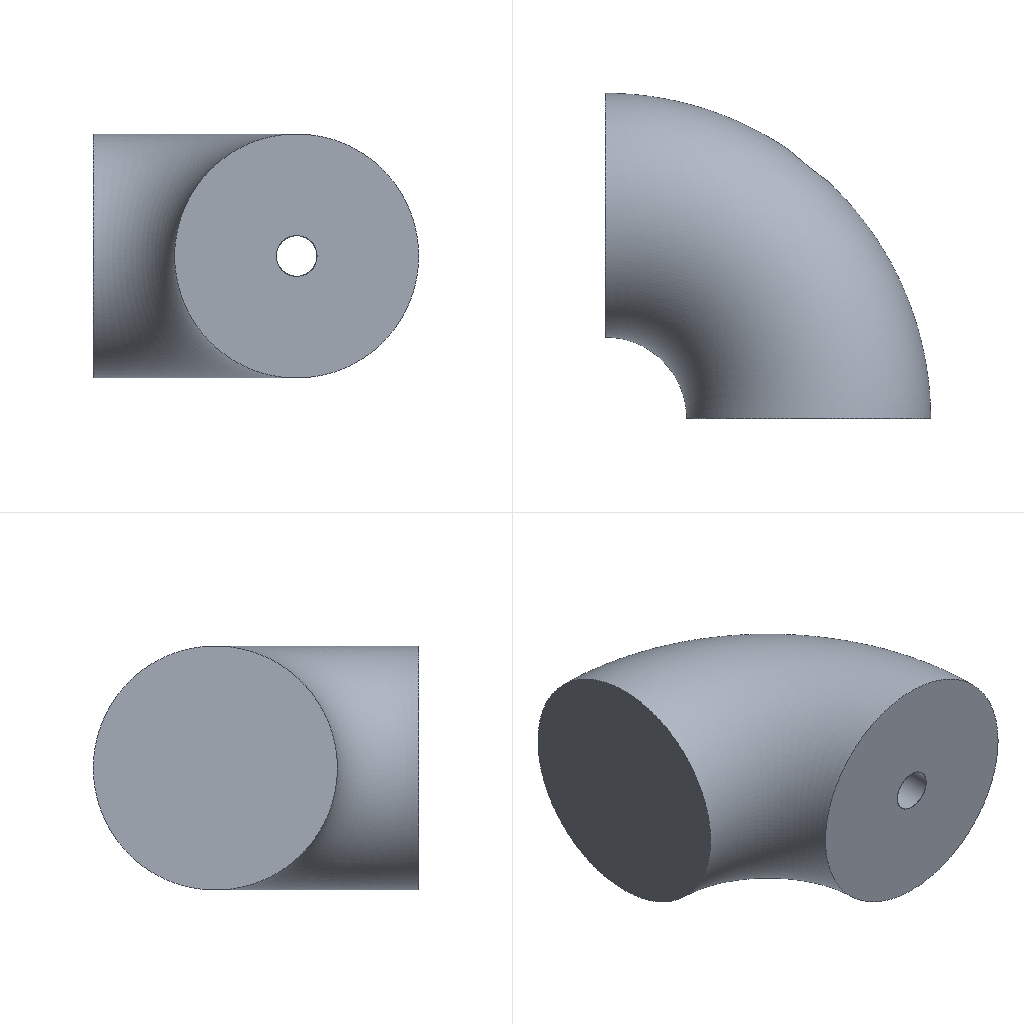Simulation study | ansys fluent
Set-up summary:
category,name,step,type,value,unit,region
solver,ansys_fluent,,Fluent 26.1.0
units,SI m-kg-s (Fluent internal),,stated,boundary values in the units shown in brackets; results in listed units
analysis,deck-1.cas,,cfd steady,"dimension=3D; solver=3d, dp, dbns imp, lam (3d, double precision, density-based implicit, laminar); source_case=2.cas"
model,Space,deck-1.cas,,3D
model,Time,deck-1.cas,,Steady
model,Viscous,deck-1.cas,,Laminar
model,Heat Transfer,deck-1.cas,,Enabled
model,Multiphase,deck-1.cas,,Disabled
analysis,deck-2.cas,,cfd steady,"dimension=3D; solver=3d, dp, dbns imp, lam (3d, double precision, density-based implicit, laminar); source_case=.cas.h5"
model,Space,deck-2.cas,,3D
model,Time,deck-2.cas,,Steady
model,Viscous,deck-2.cas,,Laminar
model,Heat Transfer,deck-2.cas,,Enabled
model,Multiphase,deck-2.cas,,Disabled
mesh,deck-1.cas,,nodes,282132
mesh,deck-1.cas,,elements,266016
mesh,deck-1.cas,,faces,813961
mesh,deck-1.cas,,note,elements = cells; counts from the case file zone headers
mesh,deck-2.cas,,nodes,282132
mesh,deck-2.cas,,elements,266016
mesh,deck-2.cas,,faces,813961
mesh,deck-2.cas,,note,elements = cells; counts from the case file zone headers
cell_zone,fluid,deck-1.cas,fluid,material=air,,zone 11
cell_zone,fluid,deck-2.cas,fluid,material=air,,zone 11
material,air (fluid),,Density,1.225,kg/m^3
material,air (fluid),,Cp (Specific Heat),1006.43,J/(kg K)
material,air (fluid),,Thermal Conductivity,0.0242,W/(m K)
material,air (fluid),,Viscosity,1.7894e-05,kg/(m s)
material,aluminum (solid),,Density,2719,kg/m^3
material,aluminum (solid),,Cp (Specific Heat),871,J/(kg K)
material,aluminum (solid),,Thermal Conductivity,202.4,W/(m K)
bc,out,deck-1.cas,outflow,,,zone 14
bc,in,deck-1.cas,velocity-inlet,Velocity Magnitude [m/s]=0.01,,zone 13
bc,elbow,deck-1.cas,wall,Material Name=aluminum; Thermal BC Type=Heat Flux; Wall Motion=Stationary Wall; Shear Boundary Condition=No Slip,,zone 15
bc,cylin,deck-1.cas,wall,Material Name=aluminum; Thermal BC Type=Heat Flux; Wall Motion=Stationary Wall; Shear Boundary Condition=No Slip,,zone 16
bc,out,deck-2.cas,outflow,,,zone 14
bc,in,deck-2.cas,velocity-inlet,Velocity Magnitude [m/s]=0.01,,zone 13
bc,elbow,deck-2.cas,wall,Material Name=aluminum; Thermal BC Type=Heat Flux; Wall Motion=Stationary Wall; Shear Boundary Condition=No Slip,,zone 15
bc,cylin,deck-2.cas,wall,Material Name=aluminum; Thermal BC Type=Heat Flux; Wall Motion=Stationary Wall; Shear Boundary Condition=No Slip,,zone 16
Results summary:
result,mass flow rate cylin,deck-1.cas,,-0,kg/s
result,mass flow rate elbow,deck-1.cas,,-0,kg/s
result,mass flow rate in,deck-1.cas,,0.003462,kg/s
result,mass flow rate int_fluid,deck-1.cas,,0.01102,kg/s
result,mass flow rate out,deck-1.cas,,3.21019e-18,kg/s
result,mass flow rate Net,deck-1.cas,,0.003462,kg/s
result,heat transfer rate cylin,deck-1.cas,,-2.0877e-16,W
result,heat transfer rate elbow,deck-1.cas,,1.85807e-15,W
result,heat transfer rate in,deck-1.cas,,1331.49,W
result,heat transfer rate out,deck-1.cas,,7.22059e-05,W
result,heat transfer rate Net,deck-1.cas,,1331.49,W
result,wall force total cylin,deck-1.cas,,"(1.44631e-06, -1.997e-06, -1.32931e-09)",N
result,wall force pressure cylin,deck-1.cas,,"(6.26561e-07, 1.59119e-10, -5.14845e-09)",N
result,wall force viscous cylin,deck-1.cas,,"(8.19746e-07, -1.99716e-06, 3.81914e-09)",N
result,wall force total elbow,deck-1.cas,,"(3.26671e-05, 3.23621e-05, -3.17263e-10)",N
result,wall force pressure elbow,deck-1.cas,,"(2.66046e-05, 4.0988e-05, -8.1224e-09)",N
result,wall force viscous elbow,deck-1.cas,,"(6.06255e-06, -8.6259e-06, 7.80513e-09)",N
result,wall force total Net,deck-1.cas,,"(3.41135e-05, 3.03651e-05, -1.64658e-09)",N
result,wall force pressure Net,deck-1.cas,,"(2.72312e-05, 4.09882e-05, -1.32708e-08)",N
result,wall force viscous Net,deck-1.cas,,"(6.8823e-06, -1.06231e-05, 1.16243e-08)",N
result,mass flow rate cylin,deck-2.cas,,-0,kg/s
result,mass flow rate elbow,deck-2.cas,,-0,kg/s
result,mass flow rate in,deck-2.cas,,0.003462,kg/s
result,mass flow rate int_fluid,deck-2.cas,,0.01102,kg/s
result,mass flow rate out,deck-2.cas,,3.21019e-18,kg/s
result,mass flow rate Net,deck-2.cas,,0.003462,kg/s
result,heat transfer rate cylin,deck-2.cas,,-2.0877e-16,W
result,heat transfer rate elbow,deck-2.cas,,1.85807e-15,W
result,heat transfer rate in,deck-2.cas,,1331.49,W
result,heat transfer rate out,deck-2.cas,,7.22059e-05,W
result,heat transfer rate Net,deck-2.cas,,1331.49,W
result,wall force total cylin,deck-2.cas,,"(1.44631e-06, -1.997e-06, -1.32931e-09)",N
result,wall force pressure cylin,deck-2.cas,,"(6.26561e-07, 1.59119e-10, -5.14845e-09)",N
result,wall force viscous cylin,deck-2.cas,,"(8.19746e-07, -1.99716e-06, 3.81914e-09)",N
result,wall force total elbow,deck-2.cas,,"(3.26671e-05, 3.23621e-05, -3.17263e-10)",N
result,wall force pressure elbow,deck-2.cas,,"(2.66046e-05, 4.0988e-05, -8.1224e-09)",N
result,wall force viscous elbow,deck-2.cas,,"(6.06255e-06, -8.6259e-06, 7.80513e-09)",N
result,wall force total Net,deck-2.cas,,"(3.41135e-05, 3.03651e-05, -1.64658e-09)",N
result,wall force pressure Net,deck-2.cas,,"(2.72312e-05, 4.09882e-05, -1.32708e-08)",N
result,wall force viscous Net,deck-2.cas,,"(6.8823e-06, -1.06231e-05, 1.16243e-08)",N